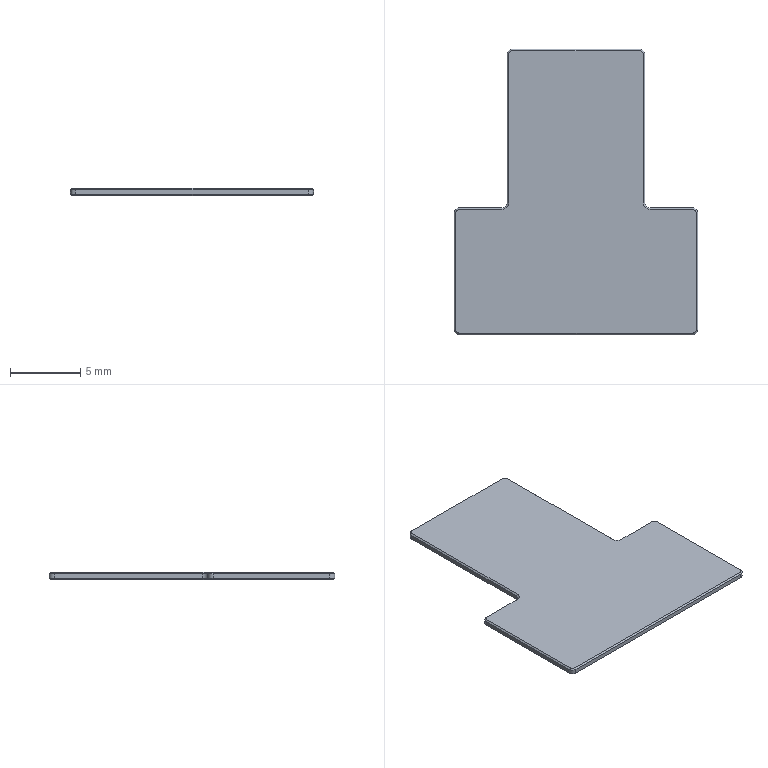Part | Creo | features DATUM PLANE 3, CHAMFER 1, COORDINATE SYSTEM 1, CURVE 1, PROTRUSION 1 | 1 solid | 50 faces | box 17.25 x 20.25 x 0.5 mm | volume 131.673 mm3 | plane 26 | cone 16 | cylinder 8 | commonest cylinder face diameters 0.75 x8
STEP:
#1=CARTESIAN_POINT('',(0.,0.,0.));
#2=DIRECTION('',(0.,0.,1.));
#3=DIRECTION('',(1.,0.,0.));
#4=AXIS2_PLACEMENT_3D('',#1,#2,#3);
#5=CARTESIAN_POINT('',(-2.122,11.783,0.));
#6=VERTEX_POINT('',#5);
#7=CARTESIAN_POINT('',(-1.847,12.058,0.));
#8=VERTEX_POINT('',#7);
#9=CARTESIAN_POINT('',(-1.847,11.783,0.));
#10=DIRECTION('',(0.,0.,-1.));
#11=DIRECTION('',(-1.,0.,0.));
#12=AXIS2_PLACEMENT_3D('',#9,#10,#11);
#13=CIRCLE('',#12,0.275);
#14=EDGE_CURVE('',#6,#8,#13,.T.);
#15=ORIENTED_EDGE('',*,*,#14,.F.);
#16=CARTESIAN_POINT('',(-2.122,1.283,0.));
#17=VERTEX_POINT('',#16);
#18=CARTESIAN_POINT('',(-2.122,1.283,0.));
#19=DIRECTION('',(0.,1.,0.));
#20=VECTOR('',#19,10.5);
#21=LINE('',#18,#20);
#22=EDGE_CURVE('',#17,#6,#21,.T.);
#23=ORIENTED_EDGE('',*,*,#22,.F.);
#24=CARTESIAN_POINT('',(-2.597,0.8081,0.000000001));
#25=VERTEX_POINT('',#24);
#26=CARTESIAN_POINT('',(-2.597,1.283,0.));
#27=DIRECTION('',(0.,0.,1.));
#28=DIRECTION('',(0.,-1.,0.));
#29=AXIS2_PLACEMENT_3D('',#26,#27,#28);
#30=CIRCLE('',#29,0.475);
#31=EDGE_CURVE('',#25,#17,#30,.T.);
#32=ORIENTED_EDGE('',*,*,#31,.F.);
#33=CARTESIAN_POINT('',(-5.597,0.8081,0.));
#34=VERTEX_POINT('',#33);
#35=CARTESIAN_POINT('',(-5.597,0.8081,-0.000000002));
#36=DIRECTION('',(1.,0.000000001,0.000000001));
#37=VECTOR('',#36,3.);
#38=LINE('',#35,#37);
#39=EDGE_CURVE('',#34,#25,#38,.T.);
#40=ORIENTED_EDGE('',*,*,#39,.F.);
#41=CARTESIAN_POINT('',(-5.872,0.5331,0.));
#42=VERTEX_POINT('',#41);
#43=CARTESIAN_POINT('',(-5.597,0.5331,0.));
#44=DIRECTION('',(0.,0.,-1.));
#45=DIRECTION('',(-1.,0.,0.));
#46=AXIS2_PLACEMENT_3D('',#43,#44,#45);
#47=CIRCLE('',#46,0.275);
#48=EDGE_CURVE('',#42,#34,#47,.T.);
#49=ORIENTED_EDGE('',*,*,#48,.F.);
#50=CARTESIAN_POINT('',(-5.872,-7.717,0.));
#51=VERTEX_POINT('',#50);
#52=CARTESIAN_POINT('',(-5.872,-7.717,-0.000000002));
#53=DIRECTION('',(0.,1.,0.));
#54=VECTOR('',#53,8.25);
#55=LINE('',#52,#54);
#56=EDGE_CURVE('',#51,#42,#55,.T.);
#57=ORIENTED_EDGE('',*,*,#56,.F.);
#58=CARTESIAN_POINT('',(-5.597,-7.992,0.));
#59=VERTEX_POINT('',#58);
#60=CARTESIAN_POINT('',(-5.597,-7.717,0.));
#61=DIRECTION('',(0.,0.,-1.));
#62=DIRECTION('',(0.,-1.,0.));
#63=AXIS2_PLACEMENT_3D('',#60,#61,#62);
#64=CIRCLE('',#63,0.275);
#65=EDGE_CURVE('',#59,#51,#64,.T.);
#66=ORIENTED_EDGE('',*,*,#65,.F.);
#67=CARTESIAN_POINT('',(10.903,-7.992,0.));
#68=VERTEX_POINT('',#67);
#69=CARTESIAN_POINT('',(10.903,-7.992,-0.000000002));
#70=DIRECTION('',(-1.,0.,0.));
#71=VECTOR('',#70,16.5);
#72=LINE('',#69,#71);
#73=EDGE_CURVE('',#68,#59,#72,.T.);
#74=ORIENTED_EDGE('',*,*,#73,.F.);
#75=CARTESIAN_POINT('',(11.178,-7.717,0.));
#76=VERTEX_POINT('',#75);
#77=CARTESIAN_POINT('',(10.903,-7.717,0.));
#78=DIRECTION('',(0.,0.,-1.));
#79=DIRECTION('',(1.,0.,0.));
#80=AXIS2_PLACEMENT_3D('',#77,#78,#79);
#81=CIRCLE('',#80,0.275);
#82=EDGE_CURVE('',#76,#68,#81,.T.);
#83=ORIENTED_EDGE('',*,*,#82,.F.);
#84=CARTESIAN_POINT('',(11.178,0.5331,0.));
#85=VERTEX_POINT('',#84);
#86=CARTESIAN_POINT('',(11.178,0.5331,-0.000000002));
#87=DIRECTION('',(0.,-1.,0.));
#88=VECTOR('',#87,8.25);
#89=LINE('',#86,#88);
#90=EDGE_CURVE('',#85,#76,#89,.T.);
#91=ORIENTED_EDGE('',*,*,#90,.F.);
#92=CARTESIAN_POINT('',(10.903,0.8081,0.));
#93=VERTEX_POINT('',#92);
#94=CARTESIAN_POINT('',(10.903,0.5331,0.));
#95=DIRECTION('',(0.,0.,-1.));
#96=DIRECTION('',(0.,1.,0.));
#97=AXIS2_PLACEMENT_3D('',#94,#95,#96);
#98=CIRCLE('',#97,0.275);
#99=EDGE_CURVE('',#93,#85,#98,.T.);
#100=ORIENTED_EDGE('',*,*,#99,.F.);
#101=CARTESIAN_POINT('',(7.903,0.8081,0.));
#102=VERTEX_POINT('',#101);
#103=CARTESIAN_POINT('',(7.903,0.8081,0.));
#104=DIRECTION('',(1.,0.,0.));
#105=VECTOR('',#104,3.);
#106=LINE('',#103,#105);
#107=EDGE_CURVE('',#102,#93,#106,.T.);
#108=ORIENTED_EDGE('',*,*,#107,.F.);
#109=CARTESIAN_POINT('',(7.428,1.283,0.000000001));
#110=VERTEX_POINT('',#109);
#111=CARTESIAN_POINT('',(7.903,1.283,0.));
#112=DIRECTION('',(0.,0.,1.));
#113=DIRECTION('',(-1.,0.,0.));
#114=AXIS2_PLACEMENT_3D('',#111,#112,#113);
#115=CIRCLE('',#114,0.475);
#116=EDGE_CURVE('',#110,#102,#115,.T.);
#117=ORIENTED_EDGE('',*,*,#116,.F.);
#118=CARTESIAN_POINT('',(7.428,11.783,0.));
#119=VERTEX_POINT('',#118);
#120=CARTESIAN_POINT('',(7.428,11.783,-0.000000002));
#121=DIRECTION('',(0.,-1.,0.));
#122=VECTOR('',#121,10.5);
#123=LINE('',#120,#122);
#124=EDGE_CURVE('',#119,#110,#123,.T.);
#125=ORIENTED_EDGE('',*,*,#124,.F.);
#126=CARTESIAN_POINT('',(7.153,12.058,0.));
#127=VERTEX_POINT('',#126);
#128=CARTESIAN_POINT('',(7.153,11.783,0.));
#129=DIRECTION('',(0.,0.,-1.));
#130=DIRECTION('',(0.,1.,0.));
#131=AXIS2_PLACEMENT_3D('',#128,#129,#130);
#132=CIRCLE('',#131,0.275);
#133=EDGE_CURVE('',#127,#119,#132,.T.);
#134=ORIENTED_EDGE('',*,*,#133,.F.);
#135=CARTESIAN_POINT('',(-1.847,12.058,-0.000000002));
#136=DIRECTION('',(1.,0.,0.));
#137=VECTOR('',#136,9.);
#138=LINE('',#135,#137);
#139=EDGE_CURVE('',#8,#127,#138,.T.);
#140=ORIENTED_EDGE('',*,*,#139,.F.);
#141=EDGE_LOOP('',(#15,#23,#32,#40,#49,#57,#66,#74,#83,#91,#100,#108,#117,#125,#134,#140));
#142=FACE_OUTER_BOUND('',#141,.F.);
#143=CARTESIAN_POINT('',(0.,0.,0.));
#144=DIRECTION('',(0.,0.,1.));
#145=DIRECTION('',(1.,0.,0.));
#146=AXIS2_PLACEMENT_3D('',#143,#144,#145);
#147=PLANE('',#146);
#148=ADVANCED_FACE('',(#142),#147,.F.);
#149=ORIENTED_EDGE('',*,*,#14,.T.);
#150=CARTESIAN_POINT('',(-1.847,12.158,0.1));
#151=VERTEX_POINT('',#150);
#152=CARTESIAN_POINT('',(-1.847,12.058,-0.000000002));
#153=DIRECTION('',(0.,0.7071,0.7071));
#154=VECTOR('',#153,0.1414);
#155=LINE('',#152,#154);
#156=EDGE_CURVE('',#8,#151,#155,.T.);
#157=ORIENTED_EDGE('',*,*,#156,.T.);
#158=CARTESIAN_POINT('',(-2.222,11.783,0.1));
#159=VERTEX_POINT('',#158);
#160=CARTESIAN_POINT('',(-1.847,11.783,0.1));
#161=DIRECTION('',(0.,0.,-1.));
#162=DIRECTION('',(-1.,0.,0.));
#163=AXIS2_PLACEMENT_3D('',#160,#161,#162);
#164=CIRCLE('',#163,0.375);
#165=EDGE_CURVE('',#159,#151,#164,.T.);
#166=ORIENTED_EDGE('',*,*,#165,.F.);
#167=CARTESIAN_POINT('',(-2.122,11.783,0.));
#168=DIRECTION('',(-0.7071,0.,0.7071));
#169=VECTOR('',#168,0.1414);
#170=LINE('',#167,#169);
#171=EDGE_CURVE('',#6,#159,#170,.T.);
#172=ORIENTED_EDGE('',*,*,#171,.F.);
#173=EDGE_LOOP('',(#149,#157,#166,#172));
#174=FACE_OUTER_BOUND('',#173,.F.);
#175=CARTESIAN_POINT('',(-1.847,11.783,0.05));
#176=DIRECTION('',(0.,0.,1.));
#177=DIRECTION('',(0.,-1.,0.));
#178=AXIS2_PLACEMENT_3D('',#175,#176,#177);
#179=CONICAL_SURFACE('',#178,0.325,45.);
#180=ADVANCED_FACE('',(#174),#179,.T.);
#181=ORIENTED_EDGE('',*,*,#139,.T.);
#182=CARTESIAN_POINT('',(7.153,12.158,0.1));
#183=VERTEX_POINT('',#182);
#184=CARTESIAN_POINT('',(7.153,12.058,0.));
#185=DIRECTION('',(0.,0.7071,0.7071));
#186=VECTOR('',#185,0.1414);
#187=LINE('',#184,#186);
#188=EDGE_CURVE('',#127,#183,#187,.T.);
#189=ORIENTED_EDGE('',*,*,#188,.T.);
#190=CARTESIAN_POINT('',(-1.847,12.158,0.1));
#191=DIRECTION('',(1.,0.,0.));
#192=VECTOR('',#191,9.);
#193=LINE('',#190,#192);
#194=EDGE_CURVE('',#151,#183,#193,.T.);
#195=ORIENTED_EDGE('',*,*,#194,.F.);
#196=ORIENTED_EDGE('',*,*,#156,.F.);
#197=EDGE_LOOP('',(#181,#189,#195,#196));
#198=FACE_OUTER_BOUND('',#197,.F.);
#199=CARTESIAN_POINT('',(2.653,12.108,0.05));
#200=DIRECTION('',(0.,0.7071,-0.7071));
#201=DIRECTION('',(0.,0.7071,0.7071));
#202=AXIS2_PLACEMENT_3D('',#199,#200,#201);
#203=PLANE('',#202);
#204=ADVANCED_FACE('',(#198),#203,.T.);
#205=ORIENTED_EDGE('',*,*,#133,.T.);
#206=CARTESIAN_POINT('',(7.528,11.783,0.1));
#207=VERTEX_POINT('',#206);
#208=CARTESIAN_POINT('',(7.428,11.783,-0.000000002));
#209=DIRECTION('',(0.7071,0.,0.7071));
#210=VECTOR('',#209,0.1414);
#211=LINE('',#208,#210);
#212=EDGE_CURVE('',#119,#207,#211,.T.);
#213=ORIENTED_EDGE('',*,*,#212,.T.);
#214=CARTESIAN_POINT('',(7.153,11.783,0.1));
#215=DIRECTION('',(0.,0.,-1.));
#216=DIRECTION('',(0.,1.,0.));
#217=AXIS2_PLACEMENT_3D('',#214,#215,#216);
#218=CIRCLE('',#217,0.375);
#219=EDGE_CURVE('',#183,#207,#218,.T.);
#220=ORIENTED_EDGE('',*,*,#219,.F.);
#221=ORIENTED_EDGE('',*,*,#188,.F.);
#222=EDGE_LOOP('',(#205,#213,#220,#221));
#223=FACE_OUTER_BOUND('',#222,.F.);
#224=CARTESIAN_POINT('',(7.153,11.783,0.05));
#225=DIRECTION('',(0.,0.,1.));
#226=DIRECTION('',(0.,-1.,0.));
#227=AXIS2_PLACEMENT_3D('',#224,#225,#226);
#228=CONICAL_SURFACE('',#227,0.325,45.);
#229=ADVANCED_FACE('',(#223),#228,.T.);
#230=ORIENTED_EDGE('',*,*,#124,.T.);
#231=CARTESIAN_POINT('',(7.528,1.283,0.1));
#232=VERTEX_POINT('',#231);
#233=CARTESIAN_POINT('',(7.428,1.283,0.000000001));
#234=DIRECTION('',(0.7071,0.000000023,0.7071));
#235=VECTOR('',#234,0.1414);
#236=LINE('',#233,#235);
#237=EDGE_CURVE('',#110,#232,#236,.T.);
#238=ORIENTED_EDGE('',*,*,#237,.T.);
#239=CARTESIAN_POINT('',(7.528,11.783,0.1));
#240=DIRECTION('',(0.,-1.,0.));
#241=VECTOR('',#240,10.5);
#242=LINE('',#239,#241);
#243=EDGE_CURVE('',#207,#232,#242,.T.);
#244=ORIENTED_EDGE('',*,*,#243,.F.);
#245=ORIENTED_EDGE('',*,*,#212,.F.);
#246=EDGE_LOOP('',(#230,#238,#244,#245));
#247=FACE_OUTER_BOUND('',#246,.F.);
#248=CARTESIAN_POINT('',(7.478,6.533,0.05));
#249=DIRECTION('',(0.7071,0.,-0.7071));
#250=DIRECTION('',(0.7071,0.,0.7071));
#251=AXIS2_PLACEMENT_3D('',#248,#249,#250);
#252=PLANE('',#251);
#253=ADVANCED_FACE('',(#247),#252,.T.);
#254=ORIENTED_EDGE('',*,*,#116,.T.);
#255=CARTESIAN_POINT('',(7.903,0.9081,0.1));
#256=VERTEX_POINT('',#255);
#257=CARTESIAN_POINT('',(7.903,0.8081,0.));
#258=DIRECTION('',(0.000000001,0.7071,0.7071));
#259=VECTOR('',#258,0.1414);
#260=LINE('',#257,#259);
#261=EDGE_CURVE('',#102,#256,#260,.T.);
#262=ORIENTED_EDGE('',*,*,#261,.T.);
#263=CARTESIAN_POINT('',(7.903,1.283,0.1));
#264=DIRECTION('',(0.,0.,1.));
#265=DIRECTION('',(-1.,0.,0.));
#266=AXIS2_PLACEMENT_3D('',#263,#264,#265);
#267=CIRCLE('',#266,0.375);
#268=EDGE_CURVE('',#232,#256,#267,.T.);
#269=ORIENTED_EDGE('',*,*,#268,.F.);
#270=ORIENTED_EDGE('',*,*,#237,.F.);
#271=EDGE_LOOP('',(#254,#262,#269,#270));
#272=FACE_OUTER_BOUND('',#271,.F.);
#273=CARTESIAN_POINT('',(7.903,1.283,0.05));
#274=DIRECTION('',(0.,0.,-1.));
#275=DIRECTION('',(0.,-1.,0.));
#276=AXIS2_PLACEMENT_3D('',#273,#274,#275);
#277=CONICAL_SURFACE('',#276,0.425,45.);
#278=ADVANCED_FACE('',(#272),#277,.F.);
#279=ORIENTED_EDGE('',*,*,#107,.T.);
#280=CARTESIAN_POINT('',(10.903,0.9081,0.1));
#281=VERTEX_POINT('',#280);
#282=CARTESIAN_POINT('',(10.903,0.8081,0.));
#283=DIRECTION('',(0.,0.7071,0.7071));
#284=VECTOR('',#283,0.1414);
#285=LINE('',#282,#284);
#286=EDGE_CURVE('',#93,#281,#285,.T.);
#287=ORIENTED_EDGE('',*,*,#286,.T.);
#288=CARTESIAN_POINT('',(7.903,0.9081,0.1));
#289=DIRECTION('',(1.,0.,0.));
#290=VECTOR('',#289,3.);
#291=LINE('',#288,#290);
#292=EDGE_CURVE('',#256,#281,#291,.T.);
#293=ORIENTED_EDGE('',*,*,#292,.F.);
#294=ORIENTED_EDGE('',*,*,#261,.F.);
#295=EDGE_LOOP('',(#279,#287,#293,#294));
#296=FACE_OUTER_BOUND('',#295,.F.);
#297=CARTESIAN_POINT('',(9.403,0.8581,0.05));
#298=DIRECTION('',(0.,0.7071,-0.7071));
#299=DIRECTION('',(0.,0.7071,0.7071));
#300=AXIS2_PLACEMENT_3D('',#297,#298,#299);
#301=PLANE('',#300);
#302=ADVANCED_FACE('',(#296),#301,.T.);
#303=ORIENTED_EDGE('',*,*,#99,.T.);
#304=CARTESIAN_POINT('',(11.278,0.5331,0.1));
#305=VERTEX_POINT('',#304);
#306=CARTESIAN_POINT('',(11.178,0.5331,-0.000000002));
#307=DIRECTION('',(0.7071,0.,0.7071));
#308=VECTOR('',#307,0.1414);
#309=LINE('',#306,#308);
#310=EDGE_CURVE('',#85,#305,#309,.T.);
#311=ORIENTED_EDGE('',*,*,#310,.T.);
#312=CARTESIAN_POINT('',(10.903,0.5331,0.1));
#313=DIRECTION('',(0.,0.,-1.));
#314=DIRECTION('',(0.,1.,0.));
#315=AXIS2_PLACEMENT_3D('',#312,#313,#314);
#316=CIRCLE('',#315,0.375);
#317=EDGE_CURVE('',#281,#305,#316,.T.);
#318=ORIENTED_EDGE('',*,*,#317,.F.);
#319=ORIENTED_EDGE('',*,*,#286,.F.);
#320=EDGE_LOOP('',(#303,#311,#318,#319));
#321=FACE_OUTER_BOUND('',#320,.F.);
#322=CARTESIAN_POINT('',(10.903,0.5331,0.05));
#323=DIRECTION('',(0.,0.,1.));
#324=DIRECTION('',(0.,-1.,0.));
#325=AXIS2_PLACEMENT_3D('',#322,#323,#324);
#326=CONICAL_SURFACE('',#325,0.325,45.);
#327=ADVANCED_FACE('',(#321),#326,.T.);
#328=ORIENTED_EDGE('',*,*,#90,.T.);
#329=CARTESIAN_POINT('',(11.278,-7.717,0.1));
#330=VERTEX_POINT('',#329);
#331=CARTESIAN_POINT('',(11.178,-7.717,0.));
#332=DIRECTION('',(0.7071,0.,0.7071));
#333=VECTOR('',#332,0.1414);
#334=LINE('',#331,#333);
#335=EDGE_CURVE('',#76,#330,#334,.T.);
#336=ORIENTED_EDGE('',*,*,#335,.T.);
#337=CARTESIAN_POINT('',(11.278,0.5331,0.1));
#338=DIRECTION('',(0.,-1.,0.));
#339=VECTOR('',#338,8.25);
#340=LINE('',#337,#339);
#341=EDGE_CURVE('',#305,#330,#340,.T.);
#342=ORIENTED_EDGE('',*,*,#341,.F.);
#343=ORIENTED_EDGE('',*,*,#310,.F.);
#344=EDGE_LOOP('',(#328,#336,#342,#343));
#345=FACE_OUTER_BOUND('',#344,.F.);
#346=CARTESIAN_POINT('',(11.228,-3.592,0.05));
#347=DIRECTION('',(0.7071,0.,-0.7071));
#348=DIRECTION('',(0.7071,0.,0.7071));
#349=AXIS2_PLACEMENT_3D('',#346,#347,#348);
#350=PLANE('',#349);
#351=ADVANCED_FACE('',(#345),#350,.T.);
#352=ORIENTED_EDGE('',*,*,#82,.T.);
#353=CARTESIAN_POINT('',(10.903,-8.092,0.1));
#354=VERTEX_POINT('',#353);
#355=CARTESIAN_POINT('',(10.903,-7.992,-0.000000002));
#356=DIRECTION('',(0.,-0.7071,0.7071));
#357=VECTOR('',#356,0.1414);
#358=LINE('',#355,#357);
#359=EDGE_CURVE('',#68,#354,#358,.T.);
#360=ORIENTED_EDGE('',*,*,#359,.T.);
#361=CARTESIAN_POINT('',(10.903,-7.717,0.1));
#362=DIRECTION('',(0.,0.,-1.));
#363=DIRECTION('',(1.,0.,0.));
#364=AXIS2_PLACEMENT_3D('',#361,#362,#363);
#365=CIRCLE('',#364,0.375);
#366=EDGE_CURVE('',#330,#354,#365,.T.);
#367=ORIENTED_EDGE('',*,*,#366,.F.);
#368=ORIENTED_EDGE('',*,*,#335,.F.);
#369=EDGE_LOOP('',(#352,#360,#367,#368));
#370=FACE_OUTER_BOUND('',#369,.F.);
#371=CARTESIAN_POINT('',(10.903,-7.717,0.05));
#372=DIRECTION('',(0.,0.,1.));
#373=DIRECTION('',(0.,-1.,0.));
#374=AXIS2_PLACEMENT_3D('',#371,#372,#373);
#375=CONICAL_SURFACE('',#374,0.325,45.);
#376=ADVANCED_FACE('',(#370),#375,.T.);
#377=ORIENTED_EDGE('',*,*,#73,.T.);
#378=CARTESIAN_POINT('',(-5.597,-8.092,0.1));
#379=VERTEX_POINT('',#378);
#380=CARTESIAN_POINT('',(-5.597,-7.992,0.));
#381=DIRECTION('',(0.,-0.7071,0.7071));
#382=VECTOR('',#381,0.1414);
#383=LINE('',#380,#382);
#384=EDGE_CURVE('',#59,#379,#383,.T.);
#385=ORIENTED_EDGE('',*,*,#384,.T.);
#386=CARTESIAN_POINT('',(10.903,-8.092,0.1));
#387=DIRECTION('',(-1.,0.,0.));
#388=VECTOR('',#387,16.5);
#389=LINE('',#386,#388);
#390=EDGE_CURVE('',#354,#379,#389,.T.);
#391=ORIENTED_EDGE('',*,*,#390,.F.);
#392=ORIENTED_EDGE('',*,*,#359,.F.);
#393=EDGE_LOOP('',(#377,#385,#391,#392));
#394=FACE_OUTER_BOUND('',#393,.F.);
#395=CARTESIAN_POINT('',(2.653,-8.042,0.05));
#396=DIRECTION('',(0.,-0.7071,-0.7071));
#397=DIRECTION('',(0.,-0.7071,0.7071));
#398=AXIS2_PLACEMENT_3D('',#395,#396,#397);
#399=PLANE('',#398);
#400=ADVANCED_FACE('',(#394),#399,.T.);
#401=ORIENTED_EDGE('',*,*,#65,.T.);
#402=CARTESIAN_POINT('',(-5.972,-7.717,0.1));
#403=VERTEX_POINT('',#402);
#404=CARTESIAN_POINT('',(-5.872,-7.717,-0.000000002));
#405=DIRECTION('',(-0.7071,0.,0.7071));
#406=VECTOR('',#405,0.1414);
#407=LINE('',#404,#406);
#408=EDGE_CURVE('',#51,#403,#407,.T.);
#409=ORIENTED_EDGE('',*,*,#408,.T.);
#410=CARTESIAN_POINT('',(-5.597,-7.717,0.1));
#411=DIRECTION('',(0.,0.,-1.));
#412=DIRECTION('',(0.,-1.,0.));
#413=AXIS2_PLACEMENT_3D('',#410,#411,#412);
#414=CIRCLE('',#413,0.375);
#415=EDGE_CURVE('',#379,#403,#414,.T.);
#416=ORIENTED_EDGE('',*,*,#415,.F.);
#417=ORIENTED_EDGE('',*,*,#384,.F.);
#418=EDGE_LOOP('',(#401,#409,#416,#417));
#419=FACE_OUTER_BOUND('',#418,.F.);
#420=CARTESIAN_POINT('',(-5.597,-7.717,0.05));
#421=DIRECTION('',(0.,0.,1.));
#422=DIRECTION('',(0.,-1.,0.));
#423=AXIS2_PLACEMENT_3D('',#420,#421,#422);
#424=CONICAL_SURFACE('',#423,0.325,45.);
#425=ADVANCED_FACE('',(#419),#424,.T.);
#426=ORIENTED_EDGE('',*,*,#56,.T.);
#427=CARTESIAN_POINT('',(-5.972,0.5331,0.1));
#428=VERTEX_POINT('',#427);
#429=CARTESIAN_POINT('',(-5.872,0.5331,0.));
#430=DIRECTION('',(-0.7071,0.,0.7071));
#431=VECTOR('',#430,0.1414);
#432=LINE('',#429,#431);
#433=EDGE_CURVE('',#42,#428,#432,.T.);
#434=ORIENTED_EDGE('',*,*,#433,.T.);
#435=CARTESIAN_POINT('',(-5.972,-7.717,0.1));
#436=DIRECTION('',(0.,1.,0.));
#437=VECTOR('',#436,8.25);
#438=LINE('',#435,#437);
#439=EDGE_CURVE('',#403,#428,#438,.T.);
#440=ORIENTED_EDGE('',*,*,#439,.F.);
#441=ORIENTED_EDGE('',*,*,#408,.F.);
#442=EDGE_LOOP('',(#426,#434,#440,#441));
#443=FACE_OUTER_BOUND('',#442,.F.);
#444=CARTESIAN_POINT('',(-5.922,-3.592,0.05));
#445=DIRECTION('',(-0.7071,0.,-0.7071));
#446=DIRECTION('',(-0.7071,0.,0.7071));
#447=AXIS2_PLACEMENT_3D('',#444,#445,#446);
#448=PLANE('',#447);
#449=ADVANCED_FACE('',(#443),#448,.T.);
#450=ORIENTED_EDGE('',*,*,#48,.T.);
#451=CARTESIAN_POINT('',(-5.597,0.9081,0.1));
#452=VERTEX_POINT('',#451);
#453=CARTESIAN_POINT('',(-5.597,0.8081,-0.000000002));
#454=DIRECTION('',(0.,0.7071,0.7071));
#455=VECTOR('',#454,0.1414);
#456=LINE('',#453,#455);
#457=EDGE_CURVE('',#34,#452,#456,.T.);
#458=ORIENTED_EDGE('',*,*,#457,.T.);
#459=CARTESIAN_POINT('',(-5.597,0.5331,0.1));
#460=DIRECTION('',(0.,0.,-1.));
#461=DIRECTION('',(-1.,0.,0.));
#462=AXIS2_PLACEMENT_3D('',#459,#460,#461);
#463=CIRCLE('',#462,0.375);
#464=EDGE_CURVE('',#428,#452,#463,.T.);
#465=ORIENTED_EDGE('',*,*,#464,.F.);
#466=ORIENTED_EDGE('',*,*,#433,.F.);
#467=EDGE_LOOP('',(#450,#458,#465,#466));
#468=FACE_OUTER_BOUND('',#467,.F.);
#469=CARTESIAN_POINT('',(-5.597,0.5331,0.05));
#470=DIRECTION('',(0.,0.,1.));
#471=DIRECTION('',(0.,-1.,0.));
#472=AXIS2_PLACEMENT_3D('',#469,#470,#471);
#473=CONICAL_SURFACE('',#472,0.325,45.);
#474=ADVANCED_FACE('',(#468),#473,.T.);
#475=ORIENTED_EDGE('',*,*,#39,.T.);
#476=CARTESIAN_POINT('',(-2.597,0.9081,0.1));
#477=VERTEX_POINT('',#476);
#478=CARTESIAN_POINT('',(-2.597,0.8081,0.000000001));
#479=DIRECTION('',(-0.000000023,0.7071,0.7071));
#480=VECTOR('',#479,0.1414);
#481=LINE('',#478,#480);
#482=EDGE_CURVE('',#25,#477,#481,.T.);
#483=ORIENTED_EDGE('',*,*,#482,.T.);
#484=CARTESIAN_POINT('',(-5.597,0.9081,0.1));
#485=DIRECTION('',(1.,0.000000001,0.000000001));
#486=VECTOR('',#485,3.);
#487=LINE('',#484,#486);
#488=EDGE_CURVE('',#452,#477,#487,.T.);
#489=ORIENTED_EDGE('',*,*,#488,.F.);
#490=ORIENTED_EDGE('',*,*,#457,.F.);
#491=EDGE_LOOP('',(#475,#483,#489,#490));
#492=FACE_OUTER_BOUND('',#491,.F.);
#493=CARTESIAN_POINT('',(-4.097,0.8581,0.05));
#494=DIRECTION('',(0.,0.7071,-0.7071));
#495=DIRECTION('',(0.,0.7071,0.7071));
#496=AXIS2_PLACEMENT_3D('',#493,#494,#495);
#497=PLANE('',#496);
#498=ADVANCED_FACE('',(#492),#497,.T.);
#499=ORIENTED_EDGE('',*,*,#31,.T.);
#500=CARTESIAN_POINT('',(-2.222,1.283,0.1));
#501=VERTEX_POINT('',#500);
#502=CARTESIAN_POINT('',(-2.122,1.283,0.));
#503=DIRECTION('',(-0.7071,0.000000001,0.7071));
#504=VECTOR('',#503,0.1414);
#505=LINE('',#502,#504);
#506=EDGE_CURVE('',#17,#501,#505,.T.);
#507=ORIENTED_EDGE('',*,*,#506,.T.);
#508=CARTESIAN_POINT('',(-2.597,1.283,0.1));
#509=DIRECTION('',(0.,0.,1.));
#510=DIRECTION('',(0.,-1.,0.));
#511=AXIS2_PLACEMENT_3D('',#508,#509,#510);
#512=CIRCLE('',#511,0.375);
#513=EDGE_CURVE('',#477,#501,#512,.T.);
#514=ORIENTED_EDGE('',*,*,#513,.F.);
#515=ORIENTED_EDGE('',*,*,#482,.F.);
#516=EDGE_LOOP('',(#499,#507,#514,#515));
#517=FACE_OUTER_BOUND('',#516,.F.);
#518=CARTESIAN_POINT('',(-2.597,1.283,0.05));
#519=DIRECTION('',(0.,0.,-1.));
#520=DIRECTION('',(0.,-1.,0.));
#521=AXIS2_PLACEMENT_3D('',#518,#519,#520);
#522=CONICAL_SURFACE('',#521,0.425,45.);
#523=ADVANCED_FACE('',(#517),#522,.F.);
#524=ORIENTED_EDGE('',*,*,#22,.T.);
#525=ORIENTED_EDGE('',*,*,#171,.T.);
#526=CARTESIAN_POINT('',(-2.222,1.283,0.1));
#527=DIRECTION('',(0.,1.,0.));
#528=VECTOR('',#527,10.5);
#529=LINE('',#526,#528);
#530=EDGE_CURVE('',#501,#159,#529,.T.);
#531=ORIENTED_EDGE('',*,*,#530,.F.);
#532=ORIENTED_EDGE('',*,*,#506,.F.);
#533=EDGE_LOOP('',(#524,#525,#531,#532));
#534=FACE_OUTER_BOUND('',#533,.F.);
#535=CARTESIAN_POINT('',(-2.172,6.533,0.05));
#536=DIRECTION('',(-0.7071,0.,-0.7071));
#537=DIRECTION('',(-0.7071,0.,0.7071));
#538=AXIS2_PLACEMENT_3D('',#535,#536,#537);
#539=PLANE('',#538);
#540=ADVANCED_FACE('',(#534),#539,.T.);
#541=CARTESIAN_POINT('',(-2.222,11.783,0.4));
#542=VERTEX_POINT('',#541);
#543=CARTESIAN_POINT('',(-2.222,1.283,0.4));
#544=VERTEX_POINT('',#543);
#545=CARTESIAN_POINT('',(-2.222,11.783,0.4));
#546=DIRECTION('',(0.,-1.,0.));
#547=VECTOR('',#546,10.5);
#548=LINE('',#545,#547);
#549=EDGE_CURVE('',#542,#544,#548,.T.);
#550=ORIENTED_EDGE('',*,*,#549,.T.);
#551=CARTESIAN_POINT('',(-2.222,1.283,0.1));
#552=DIRECTION('',(0.,0.,1.));
#553=VECTOR('',#552,0.3);
#554=LINE('',#551,#553);
#555=EDGE_CURVE('',#501,#544,#554,.T.);
#556=ORIENTED_EDGE('',*,*,#555,.F.);
#557=ORIENTED_EDGE('',*,*,#530,.T.);
#558=CARTESIAN_POINT('',(-2.222,11.783,0.1));
#559=DIRECTION('',(0.,0.,1.));
#560=VECTOR('',#559,0.3);
#561=LINE('',#558,#560);
#562=EDGE_CURVE('',#159,#542,#561,.T.);
#563=ORIENTED_EDGE('',*,*,#562,.T.);
#564=EDGE_LOOP('',(#550,#556,#557,#563));
#565=FACE_OUTER_BOUND('',#564,.F.);
#566=CARTESIAN_POINT('',(-2.222,11.783,0.));
#567=DIRECTION('',(-1.,0.,0.));
#568=DIRECTION('',(0.,-1.,0.));
#569=AXIS2_PLACEMENT_3D('',#566,#567,#568);
#570=PLANE('',#569);
#571=ADVANCED_FACE('',(#565),#570,.T.);
#572=CARTESIAN_POINT('',(-2.122,11.783,0.5));
#573=VERTEX_POINT('',#572);
#574=CARTESIAN_POINT('',(-2.122,1.283,0.5));
#575=VERTEX_POINT('',#574);
#576=CARTESIAN_POINT('',(-2.122,11.783,0.5));
#577=DIRECTION('',(0.,-1.,0.));
#578=VECTOR('',#577,10.5);
#579=LINE('',#576,#578);
#580=EDGE_CURVE('',#573,#575,#579,.T.);
#581=ORIENTED_EDGE('',*,*,#580,.T.);
#582=CARTESIAN_POINT('',(-2.122,1.283,0.5));
#583=DIRECTION('',(-0.7071,0.000000001,-0.7071));
#584=VECTOR('',#583,0.1414);
#585=LINE('',#582,#584);
#586=EDGE_CURVE('',#575,#544,#585,.T.);
#587=ORIENTED_EDGE('',*,*,#586,.T.);
#588=ORIENTED_EDGE('',*,*,#549,.F.);
#589=CARTESIAN_POINT('',(-2.122,11.783,0.5));
#590=DIRECTION('',(-0.7071,0.,-0.7071));
#591=VECTOR('',#590,0.1414);
#592=LINE('',#589,#591);
#593=EDGE_CURVE('',#573,#542,#592,.T.);
#594=ORIENTED_EDGE('',*,*,#593,.F.);
#595=EDGE_LOOP('',(#581,#587,#588,#594));
#596=FACE_OUTER_BOUND('',#595,.F.);
#597=CARTESIAN_POINT('',(-2.172,6.533,0.45));
#598=DIRECTION('',(-0.7071,0.,0.7071));
#599=DIRECTION('',(-0.7071,0.,-0.7071));
#600=AXIS2_PLACEMENT_3D('',#597,#598,#599);
#601=PLANE('',#600);
#602=ADVANCED_FACE('',(#596),#601,.T.);
#603=CARTESIAN_POINT('',(-2.597,0.8081,0.5));
#604=VERTEX_POINT('',#603);
#605=CARTESIAN_POINT('',(-2.597,1.283,0.5));
#606=DIRECTION('',(0.,0.,-1.));
#607=DIRECTION('',(1.,0.,0.));
#608=AXIS2_PLACEMENT_3D('',#605,#606,#607);
#609=CIRCLE('',#608,0.475);
#610=EDGE_CURVE('',#575,#604,#609,.T.);
#611=ORIENTED_EDGE('',*,*,#610,.F.);
#612=ORIENTED_EDGE('',*,*,#580,.F.);
#613=CARTESIAN_POINT('',(-1.847,12.058,0.5));
#614=VERTEX_POINT('',#613);
#615=CARTESIAN_POINT('',(-1.847,11.783,0.5));
#616=DIRECTION('',(0.,0.,1.));
#617=DIRECTION('',(0.,1.,0.));
#618=AXIS2_PLACEMENT_3D('',#615,#616,#617);
#619=CIRCLE('',#618,0.275);
#620=EDGE_CURVE('',#614,#573,#619,.T.);
#621=ORIENTED_EDGE('',*,*,#620,.F.);
#622=CARTESIAN_POINT('',(7.153,12.058,0.5));
#623=VERTEX_POINT('',#622);
#624=CARTESIAN_POINT('',(7.153,12.058,0.5));
#625=DIRECTION('',(-1.,0.,0.));
#626=VECTOR('',#625,9.);
#627=LINE('',#624,#626);
#628=EDGE_CURVE('',#623,#614,#627,.T.);
#629=ORIENTED_EDGE('',*,*,#628,.F.);
#630=CARTESIAN_POINT('',(7.428,11.783,0.5));
#631=VERTEX_POINT('',#630);
#632=CARTESIAN_POINT('',(7.153,11.783,0.5));
#633=DIRECTION('',(0.,0.,1.));
#634=DIRECTION('',(1.,0.,0.));
#635=AXIS2_PLACEMENT_3D('',#632,#633,#634);
#636=CIRCLE('',#635,0.275);
#637=EDGE_CURVE('',#631,#623,#636,.T.);
#638=ORIENTED_EDGE('',*,*,#637,.F.);
#639=CARTESIAN_POINT('',(7.428,1.283,0.5));
#640=VERTEX_POINT('',#639);
#641=CARTESIAN_POINT('',(7.428,1.283,0.5));
#642=DIRECTION('',(0.,1.,0.));
#643=VECTOR('',#642,10.5);
#644=LINE('',#641,#643);
#645=EDGE_CURVE('',#640,#631,#644,.T.);
#646=ORIENTED_EDGE('',*,*,#645,.F.);
#647=CARTESIAN_POINT('',(7.903,0.8081,0.5));
#648=VERTEX_POINT('',#647);
#649=CARTESIAN_POINT('',(7.903,1.283,0.5));
#650=DIRECTION('',(0.,0.,-1.));
#651=DIRECTION('',(0.,-1.,0.));
#652=AXIS2_PLACEMENT_3D('',#649,#650,#651);
#653=CIRCLE('',#652,0.475);
#654=EDGE_CURVE('',#648,#640,#653,.T.);
#655=ORIENTED_EDGE('',*,*,#654,.F.);
#656=CARTESIAN_POINT('',(10.903,0.8081,0.5));
#657=VERTEX_POINT('',#656);
#658=CARTESIAN_POINT('',(10.903,0.8081,0.5));
#659=DIRECTION('',(-1.,0.,0.));
#660=VECTOR('',#659,3.);
#661=LINE('',#658,#660);
#662=EDGE_CURVE('',#657,#648,#661,.T.);
#663=ORIENTED_EDGE('',*,*,#662,.F.);
#664=CARTESIAN_POINT('',(11.178,0.5331,0.5));
#665=VERTEX_POINT('',#664);
#666=CARTESIAN_POINT('',(10.903,0.5331,0.5));
#667=DIRECTION('',(0.,0.,1.));
#668=DIRECTION('',(1.,0.,0.));
#669=AXIS2_PLACEMENT_3D('',#666,#667,#668);
#670=CIRCLE('',#669,0.275);
#671=EDGE_CURVE('',#665,#657,#670,.T.);
#672=ORIENTED_EDGE('',*,*,#671,.F.);
#673=CARTESIAN_POINT('',(11.178,-7.717,0.5));
#674=VERTEX_POINT('',#673);
#675=CARTESIAN_POINT('',(11.178,-7.717,0.5));
#676=DIRECTION('',(0.,1.,0.));
#677=VECTOR('',#676,8.25);
#678=LINE('',#675,#677);
#679=EDGE_CURVE('',#674,#665,#678,.T.);
#680=ORIENTED_EDGE('',*,*,#679,.F.);
#681=CARTESIAN_POINT('',(10.903,-7.992,0.5));
#682=VERTEX_POINT('',#681);
#683=CARTESIAN_POINT('',(10.903,-7.717,0.5));
#684=DIRECTION('',(0.,0.,1.));
#685=DIRECTION('',(0.,-1.,0.));
#686=AXIS2_PLACEMENT_3D('',#683,#684,#685);
#687=CIRCLE('',#686,0.275);
#688=EDGE_CURVE('',#682,#674,#687,.T.);
#689=ORIENTED_EDGE('',*,*,#688,.F.);
#690=CARTESIAN_POINT('',(-5.597,-7.992,0.5));
#691=VERTEX_POINT('',#690);
#692=CARTESIAN_POINT('',(-5.597,-7.992,0.5));
#693=DIRECTION('',(1.,0.,0.));
#694=VECTOR('',#693,16.5);
#695=LINE('',#692,#694);
#696=EDGE_CURVE('',#691,#682,#695,.T.);
#697=ORIENTED_EDGE('',*,*,#696,.F.);
#698=CARTESIAN_POINT('',(-5.872,-7.717,0.5));
#699=VERTEX_POINT('',#698);
#700=CARTESIAN_POINT('',(-5.597,-7.717,0.5));
#701=DIRECTION('',(0.,0.,1.));
#702=DIRECTION('',(-1.,0.,0.));
#703=AXIS2_PLACEMENT_3D('',#700,#701,#702);
#704=CIRCLE('',#703,0.275);
#705=EDGE_CURVE('',#699,#691,#704,.T.);
#706=ORIENTED_EDGE('',*,*,#705,.F.);
#707=CARTESIAN_POINT('',(-5.872,0.5331,0.5));
#708=VERTEX_POINT('',#707);
#709=CARTESIAN_POINT('',(-5.872,0.5331,0.5));
#710=DIRECTION('',(0.,-1.,0.));
#711=VECTOR('',#710,8.25);
#712=LINE('',#709,#711);
#713=EDGE_CURVE('',#708,#699,#712,.T.);
#714=ORIENTED_EDGE('',*,*,#713,.F.);
#715=CARTESIAN_POINT('',(-5.597,0.8081,0.5));
#716=VERTEX_POINT('',#715);
#717=CARTESIAN_POINT('',(-5.597,0.5331,0.5));
#718=DIRECTION('',(0.,0.,1.));
#719=DIRECTION('',(0.,1.,0.));
#720=AXIS2_PLACEMENT_3D('',#717,#718,#719);
#721=CIRCLE('',#720,0.275);
#722=EDGE_CURVE('',#716,#708,#721,.T.);
#723=ORIENTED_EDGE('',*,*,#722,.F.);
#724=CARTESIAN_POINT('',(-2.597,0.8081,0.5));
#725=DIRECTION('',(-1.,-0.000000001,0.000000001));
#726=VECTOR('',#725,3.);
#727=LINE('',#724,#726);
#728=EDGE_CURVE('',#604,#716,#727,.T.);
#729=ORIENTED_EDGE('',*,*,#728,.F.);
#730=EDGE_LOOP('',(#611,#612,#621,#629,#638,#646,#655,#663,#672,#680,#689,#697,#706,#714,#723,#729));
#731=FACE_OUTER_BOUND('',#730,.F.);
#732=CARTESIAN_POINT('',(0.,0.,0.5));
#733=DIRECTION('',(0.,0.,1.));
#734=DIRECTION('',(1.,0.,0.));
#735=AXIS2_PLACEMENT_3D('',#732,#733,#734);
#736=PLANE('',#735);
#737=ADVANCED_FACE('',(#731),#736,.T.);
#738=ORIENTED_EDGE('',*,*,#610,.T.);
#739=CARTESIAN_POINT('',(-2.597,0.9081,0.4));
#740=VERTEX_POINT('',#739);
#741=CARTESIAN_POINT('',(-2.597,0.8081,0.5));
#742=DIRECTION('',(-0.000000023,0.7071,-0.7071));
#743=VECTOR('',#742,0.1414);
#744=LINE('',#741,#743);
#745=EDGE_CURVE('',#604,#740,#744,.T.);
#746=ORIENTED_EDGE('',*,*,#745,.T.);
#747=CARTESIAN_POINT('',(-2.597,1.283,0.4));
#748=DIRECTION('',(0.,0.,-1.));
#749=DIRECTION('',(1.,0.,0.));
#750=AXIS2_PLACEMENT_3D('',#747,#748,#749);
#751=CIRCLE('',#750,0.375);
#752=EDGE_CURVE('',#544,#740,#751,.T.);
#753=ORIENTED_EDGE('',*,*,#752,.F.);
#754=ORIENTED_EDGE('',*,*,#586,.F.);
#755=EDGE_LOOP('',(#738,#746,#753,#754));
#756=FACE_OUTER_BOUND('',#755,.F.);
#757=CARTESIAN_POINT('',(-2.597,1.283,0.45));
#758=DIRECTION('',(0.,0.,1.));
#759=DIRECTION('',(0.,-1.,0.));
#760=AXIS2_PLACEMENT_3D('',#757,#758,#759);
#761=CONICAL_SURFACE('',#760,0.425,45.);
#762=ADVANCED_FACE('',(#756),#761,.F.);
#763=ORIENTED_EDGE('',*,*,#728,.T.);
#764=CARTESIAN_POINT('',(-5.597,0.9081,0.4));
#765=VERTEX_POINT('',#764);
#766=CARTESIAN_POINT('',(-5.597,0.8081,0.5));
#767=DIRECTION('',(0.,0.7071,-0.7071));
#768=VECTOR('',#767,0.1414);
#769=LINE('',#766,#768);
#770=EDGE_CURVE('',#716,#765,#769,.T.);
#771=ORIENTED_EDGE('',*,*,#770,.T.);
#772=CARTESIAN_POINT('',(-2.597,0.9081,0.4));
#773=DIRECTION('',(-1.,-0.000000001,0.000000001));
#774=VECTOR('',#773,3.);
#775=LINE('',#772,#774);
#776=EDGE_CURVE('',#740,#765,#775,.T.);
#777=ORIENTED_EDGE('',*,*,#776,.F.);
#778=ORIENTED_EDGE('',*,*,#745,.F.);
#779=EDGE_LOOP('',(#763,#771,#777,#778));
#780=FACE_OUTER_BOUND('',#779,.F.);
#781=CARTESIAN_POINT('',(-4.097,0.8581,0.45));
#782=DIRECTION('',(0.,0.7071,0.7071));
#783=DIRECTION('',(0.,0.7071,-0.7071));
#784=AXIS2_PLACEMENT_3D('',#781,#782,#783);
#785=PLANE('',#784);
#786=ADVANCED_FACE('',(#780),#785,.T.);
#787=ORIENTED_EDGE('',*,*,#722,.T.);
#788=CARTESIAN_POINT('',(-5.972,0.5331,0.4));
#789=VERTEX_POINT('',#788);
#790=CARTESIAN_POINT('',(-5.872,0.5331,0.5));
#791=DIRECTION('',(-0.7071,0.,-0.7071));
#792=VECTOR('',#791,0.1414);
#793=LINE('',#790,#792);
#794=EDGE_CURVE('',#708,#789,#793,.T.);
#795=ORIENTED_EDGE('',*,*,#794,.T.);
#796=CARTESIAN_POINT('',(-5.597,0.5331,0.4));
#797=DIRECTION('',(0.,0.,1.));
#798=DIRECTION('',(0.,1.,0.));
#799=AXIS2_PLACEMENT_3D('',#796,#797,#798);
#800=CIRCLE('',#799,0.375);
#801=EDGE_CURVE('',#765,#789,#800,.T.);
#802=ORIENTED_EDGE('',*,*,#801,.F.);
#803=ORIENTED_EDGE('',*,*,#770,.F.);
#804=EDGE_LOOP('',(#787,#795,#802,#803));
#805=FACE_OUTER_BOUND('',#804,.F.);
#806=CARTESIAN_POINT('',(-5.597,0.5331,0.45));
#807=DIRECTION('',(0.,0.,-1.));
#808=DIRECTION('',(0.,-1.,0.));
#809=AXIS2_PLACEMENT_3D('',#806,#807,#808);
#810=CONICAL_SURFACE('',#809,0.325,45.);
#811=ADVANCED_FACE('',(#805),#810,.T.);
#812=ORIENTED_EDGE('',*,*,#713,.T.);
#813=CARTESIAN_POINT('',(-5.972,-7.717,0.4));
#814=VERTEX_POINT('',#813);
#815=CARTESIAN_POINT('',(-5.872,-7.717,0.5));
#816=DIRECTION('',(-0.7071,0.,-0.7071));
#817=VECTOR('',#816,0.1414);
#818=LINE('',#815,#817);
#819=EDGE_CURVE('',#699,#814,#818,.T.);
#820=ORIENTED_EDGE('',*,*,#819,.T.);
#821=CARTESIAN_POINT('',(-5.972,0.5331,0.4));
#822=DIRECTION('',(0.,-1.,0.));
#823=VECTOR('',#822,8.25);
#824=LINE('',#821,#823);
#825=EDGE_CURVE('',#789,#814,#824,.T.);
#826=ORIENTED_EDGE('',*,*,#825,.F.);
#827=ORIENTED_EDGE('',*,*,#794,.F.);
#828=EDGE_LOOP('',(#812,#820,#826,#827));
#829=FACE_OUTER_BOUND('',#828,.F.);
#830=CARTESIAN_POINT('',(-5.922,-3.592,0.45));
#831=DIRECTION('',(-0.7071,0.,0.7071));
#832=DIRECTION('',(-0.7071,0.,-0.7071));
#833=AXIS2_PLACEMENT_3D('',#830,#831,#832);
#834=PLANE('',#833);
#835=ADVANCED_FACE('',(#829),#834,.T.);
#836=ORIENTED_EDGE('',*,*,#705,.T.);
#837=CARTESIAN_POINT('',(-5.597,-8.092,0.4));
#838=VERTEX_POINT('',#837);
#839=CARTESIAN_POINT('',(-5.597,-7.992,0.5));
#840=DIRECTION('',(0.,-0.7071,-0.7071));
#841=VECTOR('',#840,0.1414);
#842=LINE('',#839,#841);
#843=EDGE_CURVE('',#691,#838,#842,.T.);
#844=ORIENTED_EDGE('',*,*,#843,.T.);
#845=CARTESIAN_POINT('',(-5.597,-7.717,0.4));
#846=DIRECTION('',(0.,0.,1.));
#847=DIRECTION('',(-1.,0.,0.));
#848=AXIS2_PLACEMENT_3D('',#845,#846,#847);
#849=CIRCLE('',#848,0.375);
#850=EDGE_CURVE('',#814,#838,#849,.T.);
#851=ORIENTED_EDGE('',*,*,#850,.F.);
#852=ORIENTED_EDGE('',*,*,#819,.F.);
#853=EDGE_LOOP('',(#836,#844,#851,#852));
#854=FACE_OUTER_BOUND('',#853,.F.);
#855=CARTESIAN_POINT('',(-5.597,-7.717,0.45));
#856=DIRECTION('',(0.,0.,-1.));
#857=DIRECTION('',(0.,-1.,0.));
#858=AXIS2_PLACEMENT_3D('',#855,#856,#857);
#859=CONICAL_SURFACE('',#858,0.325,45.);
#860=ADVANCED_FACE('',(#854),#859,.T.);
#861=ORIENTED_EDGE('',*,*,#696,.T.);
#862=CARTESIAN_POINT('',(10.903,-8.092,0.4));
#863=VERTEX_POINT('',#862);
#864=CARTESIAN_POINT('',(10.903,-7.992,0.5));
#865=DIRECTION('',(0.,-0.7071,-0.7071));
#866=VECTOR('',#865,0.1414);
#867=LINE('',#864,#866);
#868=EDGE_CURVE('',#682,#863,#867,.T.);
#869=ORIENTED_EDGE('',*,*,#868,.T.);
#870=CARTESIAN_POINT('',(-5.597,-8.092,0.4));
#871=DIRECTION('',(1.,0.,0.));
#872=VECTOR('',#871,16.5);
#873=LINE('',#870,#872);
#874=EDGE_CURVE('',#838,#863,#873,.T.);
#875=ORIENTED_EDGE('',*,*,#874,.F.);
#876=ORIENTED_EDGE('',*,*,#843,.F.);
#877=EDGE_LOOP('',(#861,#869,#875,#876));
#878=FACE_OUTER_BOUND('',#877,.F.);
#879=CARTESIAN_POINT('',(2.653,-8.042,0.45));
#880=DIRECTION('',(0.,-0.7071,0.7071));
#881=DIRECTION('',(0.,-0.7071,-0.7071));
#882=AXIS2_PLACEMENT_3D('',#879,#880,#881);
#883=PLANE('',#882);
#884=ADVANCED_FACE('',(#878),#883,.T.);
#885=ORIENTED_EDGE('',*,*,#688,.T.);
#886=CARTESIAN_POINT('',(11.278,-7.717,0.4));
#887=VERTEX_POINT('',#886);
#888=CARTESIAN_POINT('',(11.178,-7.717,0.5));
#889=DIRECTION('',(0.7071,0.,-0.7071));
#890=VECTOR('',#889,0.1414);
#891=LINE('',#888,#890);
#892=EDGE_CURVE('',#674,#887,#891,.T.);
#893=ORIENTED_EDGE('',*,*,#892,.T.);
#894=CARTESIAN_POINT('',(10.903,-7.717,0.4));
#895=DIRECTION('',(0.,0.,1.));
#896=DIRECTION('',(0.,-1.,0.));
#897=AXIS2_PLACEMENT_3D('',#894,#895,#896);
#898=CIRCLE('',#897,0.375);
#899=EDGE_CURVE('',#863,#887,#898,.T.);
#900=ORIENTED_EDGE('',*,*,#899,.F.);
#901=ORIENTED_EDGE('',*,*,#868,.F.);
#902=EDGE_LOOP('',(#885,#893,#900,#901));
#903=FACE_OUTER_BOUND('',#902,.F.);
#904=CARTESIAN_POINT('',(10.903,-7.717,0.45));
#905=DIRECTION('',(0.,0.,-1.));
#906=DIRECTION('',(0.,-1.,0.));
#907=AXIS2_PLACEMENT_3D('',#904,#905,#906);
#908=CONICAL_SURFACE('',#907,0.325,45.);
#909=ADVANCED_FACE('',(#903),#908,.T.);
#910=ORIENTED_EDGE('',*,*,#679,.T.);
#911=CARTESIAN_POINT('',(11.278,0.5331,0.4));
#912=VERTEX_POINT('',#911);
#913=CARTESIAN_POINT('',(11.178,0.5331,0.5));
#914=DIRECTION('',(0.7071,0.,-0.7071));
#915=VECTOR('',#914,0.1414);
#916=LINE('',#913,#915);
#917=EDGE_CURVE('',#665,#912,#916,.T.);
#918=ORIENTED_EDGE('',*,*,#917,.T.);
#919=CARTESIAN_POINT('',(11.278,-7.717,0.4));
#920=DIRECTION('',(0.,1.,0.));
#921=VECTOR('',#920,8.25);
#922=LINE('',#919,#921);
#923=EDGE_CURVE('',#887,#912,#922,.T.);
#924=ORIENTED_EDGE('',*,*,#923,.F.);
#925=ORIENTED_EDGE('',*,*,#892,.F.);
#926=EDGE_LOOP('',(#910,#918,#924,#925));
#927=FACE_OUTER_BOUND('',#926,.F.);
#928=CARTESIAN_POINT('',(11.228,-3.592,0.45));
#929=DIRECTION('',(0.7071,0.,0.7071));
#930=DIRECTION('',(0.7071,0.,-0.7071));
#931=AXIS2_PLACEMENT_3D('',#928,#929,#930);
#932=PLANE('',#931);
#933=ADVANCED_FACE('',(#927),#932,.T.);
#934=ORIENTED_EDGE('',*,*,#671,.T.);
#935=CARTESIAN_POINT('',(10.903,0.9081,0.4));
#936=VERTEX_POINT('',#935);
#937=CARTESIAN_POINT('',(10.903,0.8081,0.5));
#938=DIRECTION('',(0.,0.7071,-0.7071));
#939=VECTOR('',#938,0.1414);
#940=LINE('',#937,#939);
#941=EDGE_CURVE('',#657,#936,#940,.T.);
#942=ORIENTED_EDGE('',*,*,#941,.T.);
#943=CARTESIAN_POINT('',(10.903,0.5331,0.4));
#944=DIRECTION('',(0.,0.,1.));
#945=DIRECTION('',(1.,0.,0.));
#946=AXIS2_PLACEMENT_3D('',#943,#944,#945);
#947=CIRCLE('',#946,0.375);
#948=EDGE_CURVE('',#912,#936,#947,.T.);
#949=ORIENTED_EDGE('',*,*,#948,.F.);
#950=ORIENTED_EDGE('',*,*,#917,.F.);
#951=EDGE_LOOP('',(#934,#942,#949,#950));
#952=FACE_OUTER_BOUND('',#951,.F.);
#953=CARTESIAN_POINT('',(10.903,0.5331,0.45));
#954=DIRECTION('',(0.,0.,-1.));
#955=DIRECTION('',(0.,-1.,0.));
#956=AXIS2_PLACEMENT_3D('',#953,#954,#955);
#957=CONICAL_SURFACE('',#956,0.325,45.);
#958=ADVANCED_FACE('',(#952),#957,.T.);
#959=ORIENTED_EDGE('',*,*,#662,.T.);
#960=CARTESIAN_POINT('',(7.903,0.9081,0.4));
#961=VERTEX_POINT('',#960);
#962=CARTESIAN_POINT('',(7.903,0.8081,0.5));
#963=DIRECTION('',(0.000000001,0.7071,-0.7071));
#964=VECTOR('',#963,0.1414);
#965=LINE('',#962,#964);
#966=EDGE_CURVE('',#648,#961,#965,.T.);
#967=ORIENTED_EDGE('',*,*,#966,.T.);
#968=CARTESIAN_POINT('',(10.903,0.9081,0.4));
#969=DIRECTION('',(-1.,0.,0.));
#970=VECTOR('',#969,3.);
#971=LINE('',#968,#970);
#972=EDGE_CURVE('',#936,#961,#971,.T.);
#973=ORIENTED_EDGE('',*,*,#972,.F.);
#974=ORIENTED_EDGE('',*,*,#941,.F.);
#975=EDGE_LOOP('',(#959,#967,#973,#974));
#976=FACE_OUTER_BOUND('',#975,.F.);
#977=CARTESIAN_POINT('',(9.403,0.8581,0.45));
#978=DIRECTION('',(0.,0.7071,0.7071));
#979=DIRECTION('',(0.,0.7071,-0.7071));
#980=AXIS2_PLACEMENT_3D('',#977,#978,#979);
#981=PLANE('',#980);
#982=ADVANCED_FACE('',(#976),#981,.T.);
#983=ORIENTED_EDGE('',*,*,#654,.T.);
#984=CARTESIAN_POINT('',(7.528,1.283,0.4));
#985=VERTEX_POINT('',#984);
#986=CARTESIAN_POINT('',(7.428,1.283,0.5));
#987=DIRECTION('',(0.7071,0.000000023,-0.7071));
#988=VECTOR('',#987,0.1414);
#989=LINE('',#986,#988);
#990=EDGE_CURVE('',#640,#985,#989,.T.);
#991=ORIENTED_EDGE('',*,*,#990,.T.);
#992=CARTESIAN_POINT('',(7.903,1.283,0.4));
#993=DIRECTION('',(0.,0.,-1.));
#994=DIRECTION('',(0.,-1.,0.));
#995=AXIS2_PLACEMENT_3D('',#992,#993,#994);
#996=CIRCLE('',#995,0.375);
#997=EDGE_CURVE('',#961,#985,#996,.T.);
#998=ORIENTED_EDGE('',*,*,#997,.F.);
#999=ORIENTED_EDGE('',*,*,#966,.F.);
#1000=EDGE_LOOP('',(#983,#991,#998,#999));
#1001=FACE_OUTER_BOUND('',#1000,.F.);
#1002=CARTESIAN_POINT('',(7.903,1.283,0.45));
#1003=DIRECTION('',(0.,0.,1.));
#1004=DIRECTION('',(0.,-1.,0.));
#1005=AXIS2_PLACEMENT_3D('',#1002,#1003,#1004);
#1006=CONICAL_SURFACE('',#1005,0.425,45.);
#1007=ADVANCED_FACE('',(#1001),#1006,.F.);
#1008=ORIENTED_EDGE('',*,*,#645,.T.);
#1009=CARTESIAN_POINT('',(7.528,11.783,0.4));
#1010=VERTEX_POINT('',#1009);
#1011=CARTESIAN_POINT('',(7.428,11.783,0.5));
#1012=DIRECTION('',(0.7071,0.,-0.7071));
#1013=VECTOR('',#1012,0.1414);
#1014=LINE('',#1011,#1013);
#1015=EDGE_CURVE('',#631,#1010,#1014,.T.);
#1016=ORIENTED_EDGE('',*,*,#1015,.T.);
#1017=CARTESIAN_POINT('',(7.528,1.283,0.4));
#1018=DIRECTION('',(0.,1.,0.));
#1019=VECTOR('',#1018,10.5);
#1020=LINE('',#1017,#1019);
#1021=EDGE_CURVE('',#985,#1010,#1020,.T.);
#1022=ORIENTED_EDGE('',*,*,#1021,.F.);
#1023=ORIENTED_EDGE('',*,*,#990,.F.);
#1024=EDGE_LOOP('',(#1008,#1016,#1022,#1023));
#1025=FACE_OUTER_BOUND('',#1024,.F.);
#1026=CARTESIAN_POINT('',(7.478,6.533,0.45));
#1027=DIRECTION('',(0.7071,0.,0.7071));
#1028=DIRECTION('',(0.7071,0.,-0.7071));
#1029=AXIS2_PLACEMENT_3D('',#1026,#1027,#1028);
#1030=PLANE('',#1029);
#1031=ADVANCED_FACE('',(#1025),#1030,.T.);
#1032=ORIENTED_EDGE('',*,*,#637,.T.);
#1033=CARTESIAN_POINT('',(7.153,12.158,0.4));
#1034=VERTEX_POINT('',#1033);
#1035=CARTESIAN_POINT('',(7.153,12.058,0.5));
#1036=DIRECTION('',(0.,0.7071,-0.7071));
#1037=VECTOR('',#1036,0.1414);
#1038=LINE('',#1035,#1037);
#1039=EDGE_CURVE('',#623,#1034,#1038,.T.);
#1040=ORIENTED_EDGE('',*,*,#1039,.T.);
#1041=CARTESIAN_POINT('',(7.153,11.783,0.4));
#1042=DIRECTION('',(0.,0.,1.));
#1043=DIRECTION('',(1.,0.,0.));
#1044=AXIS2_PLACEMENT_3D('',#1041,#1042,#1043);
#1045=CIRCLE('',#1044,0.375);
#1046=EDGE_CURVE('',#1010,#1034,#1045,.T.);
#1047=ORIENTED_EDGE('',*,*,#1046,.F.);
#1048=ORIENTED_EDGE('',*,*,#1015,.F.);
#1049=EDGE_LOOP('',(#1032,#1040,#1047,#1048));
#1050=FACE_OUTER_BOUND('',#1049,.F.);
#1051=CARTESIAN_POINT('',(7.153,11.783,0.45));
#1052=DIRECTION('',(0.,0.,-1.));
#1053=DIRECTION('',(0.,-1.,0.));
#1054=AXIS2_PLACEMENT_3D('',#1051,#1052,#1053);
#1055=CONICAL_SURFACE('',#1054,0.325,45.);
#1056=ADVANCED_FACE('',(#1050),#1055,.T.);
#1057=ORIENTED_EDGE('',*,*,#628,.T.);
#1058=CARTESIAN_POINT('',(-1.847,12.158,0.4));
#1059=VERTEX_POINT('',#1058);
#1060=CARTESIAN_POINT('',(-1.847,12.058,0.5));
#1061=DIRECTION('',(0.,0.7071,-0.7071));
#1062=VECTOR('',#1061,0.1414);
#1063=LINE('',#1060,#1062);
#1064=EDGE_CURVE('',#614,#1059,#1063,.T.);
#1065=ORIENTED_EDGE('',*,*,#1064,.T.);
#1066=CARTESIAN_POINT('',(7.153,12.158,0.4));
#1067=DIRECTION('',(-1.,0.,0.));
#1068=VECTOR('',#1067,9.);
#1069=LINE('',#1066,#1068);
#1070=EDGE_CURVE('',#1034,#1059,#1069,.T.);
#1071=ORIENTED_EDGE('',*,*,#1070,.F.);
#1072=ORIENTED_EDGE('',*,*,#1039,.F.);
#1073=EDGE_LOOP('',(#1057,#1065,#1071,#1072));
#1074=FACE_OUTER_BOUND('',#1073,.F.);
#1075=CARTESIAN_POINT('',(2.653,12.108,0.45));
#1076=DIRECTION('',(0.,0.7071,0.7071));
#1077=DIRECTION('',(0.,0.7071,-0.7071));
#1078=AXIS2_PLACEMENT_3D('',#1075,#1076,#1077);
#1079=PLANE('',#1078);
#1080=ADVANCED_FACE('',(#1074),#1079,.T.);
#1081=ORIENTED_EDGE('',*,*,#620,.T.);
#1082=ORIENTED_EDGE('',*,*,#593,.T.);
#1083=CARTESIAN_POINT('',(-1.847,11.783,0.4));
#1084=DIRECTION('',(0.,0.,1.));
#1085=DIRECTION('',(0.,1.,0.));
#1086=AXIS2_PLACEMENT_3D('',#1083,#1084,#1085);
#1087=CIRCLE('',#1086,0.375);
#1088=EDGE_CURVE('',#1059,#542,#1087,.T.);
#1089=ORIENTED_EDGE('',*,*,#1088,.F.);
#1090=ORIENTED_EDGE('',*,*,#1064,.F.);
#1091=EDGE_LOOP('',(#1081,#1082,#1089,#1090));
#1092=FACE_OUTER_BOUND('',#1091,.F.);
#1093=CARTESIAN_POINT('',(-1.847,11.783,0.45));
#1094=DIRECTION('',(0.,0.,-1.));
#1095=DIRECTION('',(0.,-1.,0.));
#1096=AXIS2_PLACEMENT_3D('',#1093,#1094,#1095);
#1097=CONICAL_SURFACE('',#1096,0.325,45.);
#1098=ADVANCED_FACE('',(#1092),#1097,.T.);
#1099=ORIENTED_EDGE('',*,*,#1088,.T.);
#1100=ORIENTED_EDGE('',*,*,#562,.F.);
#1101=ORIENTED_EDGE('',*,*,#165,.T.);
#1102=CARTESIAN_POINT('',(-1.847,12.158,0.1));
#1103=DIRECTION('',(0.,0.,1.));
#1104=VECTOR('',#1103,0.3);
#1105=LINE('',#1102,#1104);
#1106=EDGE_CURVE('',#151,#1059,#1105,.T.);
#1107=ORIENTED_EDGE('',*,*,#1106,.T.);
#1108=EDGE_LOOP('',(#1099,#1100,#1101,#1107));
#1109=FACE_OUTER_BOUND('',#1108,.F.);
#1110=CARTESIAN_POINT('',(-1.847,11.783,0.));
#1111=DIRECTION('',(0.,0.,1.));
#1112=DIRECTION('',(1.,0.,0.));
#1113=AXIS2_PLACEMENT_3D('',#1110,#1111,#1112);
#1114=CYLINDRICAL_SURFACE('',#1113,0.375);
#1115=ADVANCED_FACE('',(#1109),#1114,.T.);
#1116=ORIENTED_EDGE('',*,*,#1070,.T.);
#1117=ORIENTED_EDGE('',*,*,#1106,.F.);
#1118=ORIENTED_EDGE('',*,*,#194,.T.);
#1119=CARTESIAN_POINT('',(7.153,12.158,0.1));
#1120=DIRECTION('',(0.,0.,1.));
#1121=VECTOR('',#1120,0.3);
#1122=LINE('',#1119,#1121);
#1123=EDGE_CURVE('',#183,#1034,#1122,.T.);
#1124=ORIENTED_EDGE('',*,*,#1123,.T.);
#1125=EDGE_LOOP('',(#1116,#1117,#1118,#1124));
#1126=FACE_OUTER_BOUND('',#1125,.F.);
#1127=CARTESIAN_POINT('',(7.153,12.158,0.));
#1128=DIRECTION('',(0.,1.,0.));
#1129=DIRECTION('',(-1.,0.,0.));
#1130=AXIS2_PLACEMENT_3D('',#1127,#1128,#1129);
#1131=PLANE('',#1130);
#1132=ADVANCED_FACE('',(#1126),#1131,.T.);
#1133=ORIENTED_EDGE('',*,*,#1046,.T.);
#1134=ORIENTED_EDGE('',*,*,#1123,.F.);
#1135=ORIENTED_EDGE('',*,*,#219,.T.);
#1136=CARTESIAN_POINT('',(7.528,11.783,0.1));
#1137=DIRECTION('',(0.,0.,1.));
#1138=VECTOR('',#1137,0.3);
#1139=LINE('',#1136,#1138);
#1140=EDGE_CURVE('',#207,#1010,#1139,.T.);
#1141=ORIENTED_EDGE('',*,*,#1140,.T.);
#1142=EDGE_LOOP('',(#1133,#1134,#1135,#1141));
#1143=FACE_OUTER_BOUND('',#1142,.F.);
#1144=CARTESIAN_POINT('',(7.153,11.783,0.));
#1145=DIRECTION('',(0.,0.,1.));
#1146=DIRECTION('',(1.,0.,0.));
#1147=AXIS2_PLACEMENT_3D('',#1144,#1145,#1146);
#1148=CYLINDRICAL_SURFACE('',#1147,0.375);
#1149=ADVANCED_FACE('',(#1143),#1148,.T.);
#1150=ORIENTED_EDGE('',*,*,#1021,.T.);
#1151=ORIENTED_EDGE('',*,*,#1140,.F.);
#1152=ORIENTED_EDGE('',*,*,#243,.T.);
#1153=CARTESIAN_POINT('',(7.528,1.283,0.1));
#1154=DIRECTION('',(0.,0.,1.));
#1155=VECTOR('',#1154,0.3);
#1156=LINE('',#1153,#1155);
#1157=EDGE_CURVE('',#232,#985,#1156,.T.);
#1158=ORIENTED_EDGE('',*,*,#1157,.T.);
#1159=EDGE_LOOP('',(#1150,#1151,#1152,#1158));
#1160=FACE_OUTER_BOUND('',#1159,.F.);
#1161=CARTESIAN_POINT('',(7.528,1.283,0.));
#1162=DIRECTION('',(1.,0.,0.));
#1163=DIRECTION('',(0.,1.,0.));
#1164=AXIS2_PLACEMENT_3D('',#1161,#1162,#1163);
#1165=PLANE('',#1164);
#1166=ADVANCED_FACE('',(#1160),#1165,.T.);
#1167=ORIENTED_EDGE('',*,*,#997,.T.);
#1168=ORIENTED_EDGE('',*,*,#1157,.F.);
#1169=ORIENTED_EDGE('',*,*,#268,.T.);
#1170=CARTESIAN_POINT('',(7.903,0.9081,0.1));
#1171=DIRECTION('',(0.,0.,1.));
#1172=VECTOR('',#1171,0.3);
#1173=LINE('',#1170,#1172);
#1174=EDGE_CURVE('',#256,#961,#1173,.T.);
#1175=ORIENTED_EDGE('',*,*,#1174,.T.);
#1176=EDGE_LOOP('',(#1167,#1168,#1169,#1175));
#1177=FACE_OUTER_BOUND('',#1176,.F.);
#1178=CARTESIAN_POINT('',(7.903,1.283,0.));
#1179=DIRECTION('',(0.,0.,1.));
#1180=DIRECTION('',(1.,0.,0.));
#1181=AXIS2_PLACEMENT_3D('',#1178,#1179,#1180);
#1182=CYLINDRICAL_SURFACE('',#1181,0.375);
#1183=ADVANCED_FACE('',(#1177),#1182,.F.);
#1184=ORIENTED_EDGE('',*,*,#972,.T.);
#1185=ORIENTED_EDGE('',*,*,#1174,.F.);
#1186=ORIENTED_EDGE('',*,*,#292,.T.);
#1187=CARTESIAN_POINT('',(10.903,0.9081,0.1));
#1188=DIRECTION('',(0.,0.,1.));
#1189=VECTOR('',#1188,0.3);
#1190=LINE('',#1187,#1189);
#1191=EDGE_CURVE('',#281,#936,#1190,.T.);
#1192=ORIENTED_EDGE('',*,*,#1191,.T.);
#1193=EDGE_LOOP('',(#1184,#1185,#1186,#1192));
#1194=FACE_OUTER_BOUND('',#1193,.F.);
#1195=CARTESIAN_POINT('',(10.903,0.9081,0.));
#1196=DIRECTION('',(0.,1.,0.));
#1197=DIRECTION('',(-1.,0.,0.));
#1198=AXIS2_PLACEMENT_3D('',#1195,#1196,#1197);
#1199=PLANE('',#1198);
#1200=ADVANCED_FACE('',(#1194),#1199,.T.);
#1201=ORIENTED_EDGE('',*,*,#948,.T.);
#1202=ORIENTED_EDGE('',*,*,#1191,.F.);
#1203=ORIENTED_EDGE('',*,*,#317,.T.);
#1204=CARTESIAN_POINT('',(11.278,0.5331,0.1));
#1205=DIRECTION('',(0.,0.,1.));
#1206=VECTOR('',#1205,0.3);
#1207=LINE('',#1204,#1206);
#1208=EDGE_CURVE('',#305,#912,#1207,.T.);
#1209=ORIENTED_EDGE('',*,*,#1208,.T.);
#1210=EDGE_LOOP('',(#1201,#1202,#1203,#1209));
#1211=FACE_OUTER_BOUND('',#1210,.F.);
#1212=CARTESIAN_POINT('',(10.903,0.5331,0.));
#1213=DIRECTION('',(0.,0.,1.));
#1214=DIRECTION('',(1.,0.,0.));
#1215=AXIS2_PLACEMENT_3D('',#1212,#1213,#1214);
#1216=CYLINDRICAL_SURFACE('',#1215,0.375);
#1217=ADVANCED_FACE('',(#1211),#1216,.T.);
#1218=ORIENTED_EDGE('',*,*,#923,.T.);
#1219=ORIENTED_EDGE('',*,*,#1208,.F.);
#1220=ORIENTED_EDGE('',*,*,#341,.T.);
#1221=CARTESIAN_POINT('',(11.278,-7.717,0.1));
#1222=DIRECTION('',(0.,0.,1.));
#1223=VECTOR('',#1222,0.3);
#1224=LINE('',#1221,#1223);
#1225=EDGE_CURVE('',#330,#887,#1224,.T.);
#1226=ORIENTED_EDGE('',*,*,#1225,.T.);
#1227=EDGE_LOOP('',(#1218,#1219,#1220,#1226));
#1228=FACE_OUTER_BOUND('',#1227,.F.);
#1229=CARTESIAN_POINT('',(11.278,-7.717,0.));
#1230=DIRECTION('',(1.,0.,0.));
#1231=DIRECTION('',(0.,1.,0.));
#1232=AXIS2_PLACEMENT_3D('',#1229,#1230,#1231);
#1233=PLANE('',#1232);
#1234=ADVANCED_FACE('',(#1228),#1233,.T.);
#1235=ORIENTED_EDGE('',*,*,#899,.T.);
#1236=ORIENTED_EDGE('',*,*,#1225,.F.);
#1237=ORIENTED_EDGE('',*,*,#366,.T.);
#1238=CARTESIAN_POINT('',(10.903,-8.092,0.1));
#1239=DIRECTION('',(0.,0.,1.));
#1240=VECTOR('',#1239,0.3);
#1241=LINE('',#1238,#1240);
#1242=EDGE_CURVE('',#354,#863,#1241,.T.);
#1243=ORIENTED_EDGE('',*,*,#1242,.T.);
#1244=EDGE_LOOP('',(#1235,#1236,#1237,#1243));
#1245=FACE_OUTER_BOUND('',#1244,.F.);
#1246=CARTESIAN_POINT('',(10.903,-7.717,0.));
#1247=DIRECTION('',(0.,0.,1.));
#1248=DIRECTION('',(1.,0.,0.));
#1249=AXIS2_PLACEMENT_3D('',#1246,#1247,#1248);
#1250=CYLINDRICAL_SURFACE('',#1249,0.375);
#1251=ADVANCED_FACE('',(#1245),#1250,.T.);
#1252=ORIENTED_EDGE('',*,*,#874,.T.);
#1253=ORIENTED_EDGE('',*,*,#1242,.F.);
#1254=ORIENTED_EDGE('',*,*,#390,.T.);
#1255=CARTESIAN_POINT('',(-5.597,-8.092,0.1));
#1256=DIRECTION('',(0.,0.,1.));
#1257=VECTOR('',#1256,0.3);
#1258=LINE('',#1255,#1257);
#1259=EDGE_CURVE('',#379,#838,#1258,.T.);
#1260=ORIENTED_EDGE('',*,*,#1259,.T.);
#1261=EDGE_LOOP('',(#1252,#1253,#1254,#1260));
#1262=FACE_OUTER_BOUND('',#1261,.F.);
#1263=CARTESIAN_POINT('',(-5.597,-8.092,0.));
#1264=DIRECTION('',(0.,-1.,0.));
#1265=DIRECTION('',(1.,0.,0.));
#1266=AXIS2_PLACEMENT_3D('',#1263,#1264,#1265);
#1267=PLANE('',#1266);
#1268=ADVANCED_FACE('',(#1262),#1267,.T.);
#1269=ORIENTED_EDGE('',*,*,#850,.T.);
#1270=ORIENTED_EDGE('',*,*,#1259,.F.);
#1271=ORIENTED_EDGE('',*,*,#415,.T.);
#1272=CARTESIAN_POINT('',(-5.972,-7.717,0.1));
#1273=DIRECTION('',(0.,0.,1.));
#1274=VECTOR('',#1273,0.3);
#1275=LINE('',#1272,#1274);
#1276=EDGE_CURVE('',#403,#814,#1275,.T.);
#1277=ORIENTED_EDGE('',*,*,#1276,.T.);
#1278=EDGE_LOOP('',(#1269,#1270,#1271,#1277));
#1279=FACE_OUTER_BOUND('',#1278,.F.);
#1280=CARTESIAN_POINT('',(-5.597,-7.717,0.));
#1281=DIRECTION('',(0.,0.,1.));
#1282=DIRECTION('',(1.,0.,0.));
#1283=AXIS2_PLACEMENT_3D('',#1280,#1281,#1282);
#1284=CYLINDRICAL_SURFACE('',#1283,0.375);
#1285=ADVANCED_FACE('',(#1279),#1284,.T.);
#1286=ORIENTED_EDGE('',*,*,#825,.T.);
#1287=ORIENTED_EDGE('',*,*,#1276,.F.);
#1288=ORIENTED_EDGE('',*,*,#439,.T.);
#1289=CARTESIAN_POINT('',(-5.972,0.5331,0.1));
#1290=DIRECTION('',(0.,0.,1.));
#1291=VECTOR('',#1290,0.3);
#1292=LINE('',#1289,#1291);
#1293=EDGE_CURVE('',#428,#789,#1292,.T.);
#1294=ORIENTED_EDGE('',*,*,#1293,.T.);
#1295=EDGE_LOOP('',(#1286,#1287,#1288,#1294));
#1296=FACE_OUTER_BOUND('',#1295,.F.);
#1297=CARTESIAN_POINT('',(-5.972,0.5331,0.));
#1298=DIRECTION('',(-1.,0.,0.));
#1299=DIRECTION('',(0.,-1.,0.));
#1300=AXIS2_PLACEMENT_3D('',#1297,#1298,#1299);
#1301=PLANE('',#1300);
#1302=ADVANCED_FACE('',(#1296),#1301,.T.);
#1303=ORIENTED_EDGE('',*,*,#801,.T.);
#1304=ORIENTED_EDGE('',*,*,#1293,.F.);
#1305=ORIENTED_EDGE('',*,*,#464,.T.);
#1306=CARTESIAN_POINT('',(-5.597,0.9081,0.1));
#1307=DIRECTION('',(0.,0.,1.));
#1308=VECTOR('',#1307,0.3);
#1309=LINE('',#1306,#1308);
#1310=EDGE_CURVE('',#452,#765,#1309,.T.);
#1311=ORIENTED_EDGE('',*,*,#1310,.T.);
#1312=EDGE_LOOP('',(#1303,#1304,#1305,#1311));
#1313=FACE_OUTER_BOUND('',#1312,.F.);
#1314=CARTESIAN_POINT('',(-5.597,0.5331,0.));
#1315=DIRECTION('',(0.,0.,1.));
#1316=DIRECTION('',(1.,0.,0.));
#1317=AXIS2_PLACEMENT_3D('',#1314,#1315,#1316);
#1318=CYLINDRICAL_SURFACE('',#1317,0.375);
#1319=ADVANCED_FACE('',(#1313),#1318,.T.);
#1320=ORIENTED_EDGE('',*,*,#776,.T.);
#1321=ORIENTED_EDGE('',*,*,#1310,.F.);
#1322=ORIENTED_EDGE('',*,*,#488,.T.);
#1323=CARTESIAN_POINT('',(-2.597,0.9081,0.1));
#1324=DIRECTION('',(0.,0.,1.));
#1325=VECTOR('',#1324,0.3);
#1326=LINE('',#1323,#1325);
#1327=EDGE_CURVE('',#477,#740,#1326,.T.);
#1328=ORIENTED_EDGE('',*,*,#1327,.T.);
#1329=EDGE_LOOP('',(#1320,#1321,#1322,#1328));
#1330=FACE_OUTER_BOUND('',#1329,.F.);
#1331=CARTESIAN_POINT('',(-2.597,0.9081,0.));
#1332=DIRECTION('',(0.,1.,0.));
#1333=DIRECTION('',(-1.,0.,0.));
#1334=AXIS2_PLACEMENT_3D('',#1331,#1332,#1333);
#1335=PLANE('',#1334);
#1336=ADVANCED_FACE('',(#1330),#1335,.T.);
#1337=ORIENTED_EDGE('',*,*,#752,.T.);
#1338=ORIENTED_EDGE('',*,*,#1327,.F.);
#1339=ORIENTED_EDGE('',*,*,#513,.T.);
#1340=ORIENTED_EDGE('',*,*,#555,.T.);
#1341=EDGE_LOOP('',(#1337,#1338,#1339,#1340));
#1342=FACE_OUTER_BOUND('',#1341,.F.);
#1343=CARTESIAN_POINT('',(-2.597,1.283,0.));
#1344=DIRECTION('',(0.,0.,1.));
#1345=DIRECTION('',(1.,0.,0.));
#1346=AXIS2_PLACEMENT_3D('',#1343,#1344,#1345);
#1347=CYLINDRICAL_SURFACE('',#1346,0.375);
#1348=ADVANCED_FACE('',(#1342),#1347,.F.);
#1349=CLOSED_SHELL('',(#148,#180,#204,#229,#253,#278,#302,#327,#351,#376,#400,#425,#449,#474,#498,#523,#540,#571,#602,#737,#762,#786,#811,#835,#860,#884,#909,#933,#958,#982,#1007,#1031,#1056,#1080,#1098,#1115,#1132,#1149,#1166,#1183,#1200,#1217,#1234,#1251,#1268,#1285,#1302,#1319,#1336,#1348));
#1350=MANIFOLD_SOLID_BREP('',#1349);
#1351=(LENGTH_UNIT()NAMED_UNIT(*)SI_UNIT(.MILLI.,.METRE.));
#1352=UNCERTAINTY_MEASURE_WITH_UNIT(LENGTH_MEASURE(0.00266),#1351,'','');
#1353=(NAMED_UNIT(*)PLANE_ANGLE_UNIT()SI_UNIT($,.RADIAN.));
#1354=PLANE_ANGLE_MEASURE_WITH_UNIT(PLANE_ANGLE_MEASURE(0.01745),#1353);
#1355=(CONVERSION_BASED_UNIT('DEGREE',#1354)NAMED_UNIT(*)PLANE_ANGLE_UNIT());
#1356=(NAMED_UNIT(*)SI_UNIT($,.STERADIAN.)SOLID_ANGLE_UNIT());
#1357=(GEOMETRIC_REPRESENTATION_CONTEXT(3)GLOBAL_UNCERTAINTY_ASSIGNED_CONTEXT((#1352))GLOBAL_UNIT_ASSIGNED_CONTEXT((#1351,#1355,#1356))REPRESENTATION_CONTEXT('',''));
#1358=ADVANCED_BREP_SHAPE_REPRESENTATION('',(#4,#1350),#1357);